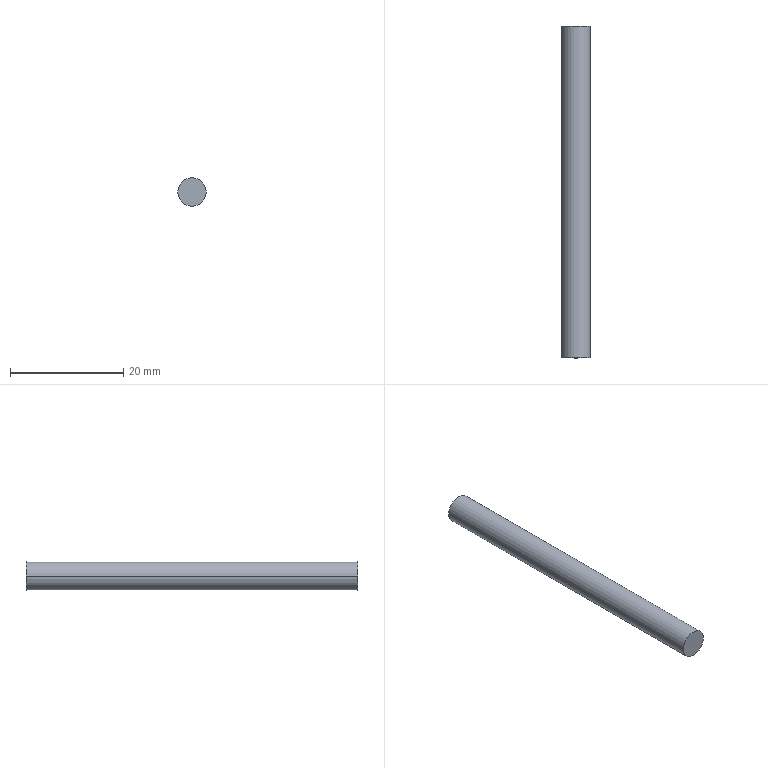Part | SolidWorks | features BaseBody 1, ICE 1 | 1 solid | 4 faces | box 5 x 58.5 x 5 mm | volume 1149 mm3 | cylinder 2 | plane 2 | commonest cylinder face diameters 5 x2
STEP:
#1=CARTESIAN_POINT('',(-2.5,249.5,188.));
#2=VERTEX_POINT('',#1);
#3=CARTESIAN_POINT('',(2.5,249.5,188.));
#4=VERTEX_POINT('',#3);
#5=CARTESIAN_POINT('',(0.,249.5,188.));
#6=DIRECTION('',(0.,-1.,0.));
#7=DIRECTION('',(0.,0.,-1.));
#8=AXIS2_PLACEMENT_3D('',#5,#6,#7);
#9=CIRCLE('',#8,2.5);
#10=EDGE_CURVE('',#2,#4,#9,.T.);
#11=ORIENTED_EDGE('',*,*,#10,.F.);
#12=CARTESIAN_POINT('',(-2.5,308.,188.));
#13=VERTEX_POINT('',#12);
#14=CARTESIAN_POINT('',(-2.5,-1127.5,188.));
#15=DIRECTION('',(0.,1.,0.));
#16=VECTOR('',#15,1000.);
#17=LINE('',#14,#16);
#18=EDGE_CURVE('',#2,#13,#17,.T.);
#19=ORIENTED_EDGE('',*,*,#18,.T.);
#20=CARTESIAN_POINT('',(2.5,308.,188.));
#21=VERTEX_POINT('',#20);
#22=CARTESIAN_POINT('',(0.,308.,188.));
#23=DIRECTION('',(0.,1.,0.));
#24=DIRECTION('',(1.,0.,0.));
#25=AXIS2_PLACEMENT_3D('',#22,#23,#24);
#26=CIRCLE('',#25,2.5);
#27=EDGE_CURVE('',#21,#13,#26,.T.);
#28=ORIENTED_EDGE('',*,*,#27,.F.);
#29=CARTESIAN_POINT('',(2.5,-1127.5,188.));
#30=DIRECTION('',(0.,1.,0.));
#31=VECTOR('',#30,1000.);
#32=LINE('',#29,#31);
#33=EDGE_CURVE('',#4,#21,#32,.T.);
#34=ORIENTED_EDGE('',*,*,#33,.F.);
#35=EDGE_LOOP('',(#11,#19,#28,#34));
#36=FACE_OUTER_BOUND('',#35,.T.);
#37=CARTESIAN_POINT('',(0.,-1127.5,188.));
#38=DIRECTION('',(0.,1.,0.));
#39=DIRECTION('',(1.,0.,0.));
#40=AXIS2_PLACEMENT_3D('',#37,#38,#39);
#41=CYLINDRICAL_SURFACE('',#40,2.5);
#42=ADVANCED_FACE('',(#36),#41,.T.);
#43=ORIENTED_EDGE('',*,*,#18,.F.);
#44=CARTESIAN_POINT('',(0.,249.5,188.));
#45=DIRECTION('',(0.,-1.,0.));
#46=DIRECTION('',(0.,0.,-1.));
#47=AXIS2_PLACEMENT_3D('',#44,#45,#46);
#48=CIRCLE('',#47,2.5);
#49=EDGE_CURVE('',#4,#2,#48,.T.);
#50=ORIENTED_EDGE('',*,*,#49,.F.);
#51=ORIENTED_EDGE('',*,*,#33,.T.);
#52=CARTESIAN_POINT('',(0.,308.,188.));
#53=DIRECTION('',(0.,1.,0.));
#54=DIRECTION('',(1.,0.,0.));
#55=AXIS2_PLACEMENT_3D('',#52,#53,#54);
#56=CIRCLE('',#55,2.5);
#57=EDGE_CURVE('',#13,#21,#56,.T.);
#58=ORIENTED_EDGE('',*,*,#57,.F.);
#59=EDGE_LOOP('',(#43,#50,#51,#58));
#60=FACE_OUTER_BOUND('',#59,.T.);
#61=CARTESIAN_POINT('',(0.,-1127.5,188.));
#62=DIRECTION('',(0.,1.,0.));
#63=DIRECTION('',(1.,0.,0.));
#64=AXIS2_PLACEMENT_3D('',#61,#62,#63);
#65=CYLINDRICAL_SURFACE('',#64,2.5);
#66=ADVANCED_FACE('',(#60),#65,.T.);
#67=ORIENTED_EDGE('',*,*,#27,.T.);
#68=ORIENTED_EDGE('',*,*,#57,.T.);
#69=EDGE_LOOP('',(#67,#68));
#70=FACE_OUTER_BOUND('',#69,.T.);
#71=CARTESIAN_POINT('',(0.,308.,188.));
#72=DIRECTION('',(0.,1.,0.));
#73=DIRECTION('',(1.,0.,0.));
#74=AXIS2_PLACEMENT_3D('',#71,#72,#73);
#75=PLANE('',#74);
#76=ADVANCED_FACE('',(#70),#75,.T.);
#77=ORIENTED_EDGE('',*,*,#49,.T.);
#78=ORIENTED_EDGE('',*,*,#10,.T.);
#79=EDGE_LOOP('',(#77,#78));
#80=FACE_OUTER_BOUND('',#79,.T.);
#81=CARTESIAN_POINT('',(0.,249.5,188.));
#82=DIRECTION('',(0.,-1.,0.));
#83=DIRECTION('',(0.,0.,-1.));
#84=AXIS2_PLACEMENT_3D('',#81,#82,#83);
#85=PLANE('',#84);
#86=ADVANCED_FACE('',(#80),#85,.T.);
#87=CLOSED_SHELL('',(#42,#66,#76,#86));
#88=MANIFOLD_SOLID_BREP('',#87);
#89=CARTESIAN_POINT('',(0.,0.,0.));
#90=DIRECTION('',(0.,0.,1.));
#91=DIRECTION('',(1.,0.,0.));
#92=AXIS2_PLACEMENT_3D('',#89,#90,#91);
#93=(LENGTH_UNIT()NAMED_UNIT(*)SI_UNIT(.MILLI.,.METRE.));
#94=UNCERTAINTY_MEASURE_WITH_UNIT(LENGTH_MEASURE(0.00001),#93,'','');
#95=(NAMED_UNIT(*)PLANE_ANGLE_UNIT()SI_UNIT($,.RADIAN.));
#96=(NAMED_UNIT(*)SI_UNIT($,.STERADIAN.)SOLID_ANGLE_UNIT());
#97=(GEOMETRIC_REPRESENTATION_CONTEXT(3)GLOBAL_UNCERTAINTY_ASSIGNED_CONTEXT((#94))GLOBAL_UNIT_ASSIGNED_CONTEXT((#93,#95,#96))REPRESENTATION_CONTEXT('',''));
#98=ADVANCED_BREP_SHAPE_REPRESENTATION('',(#88,#92),#97);